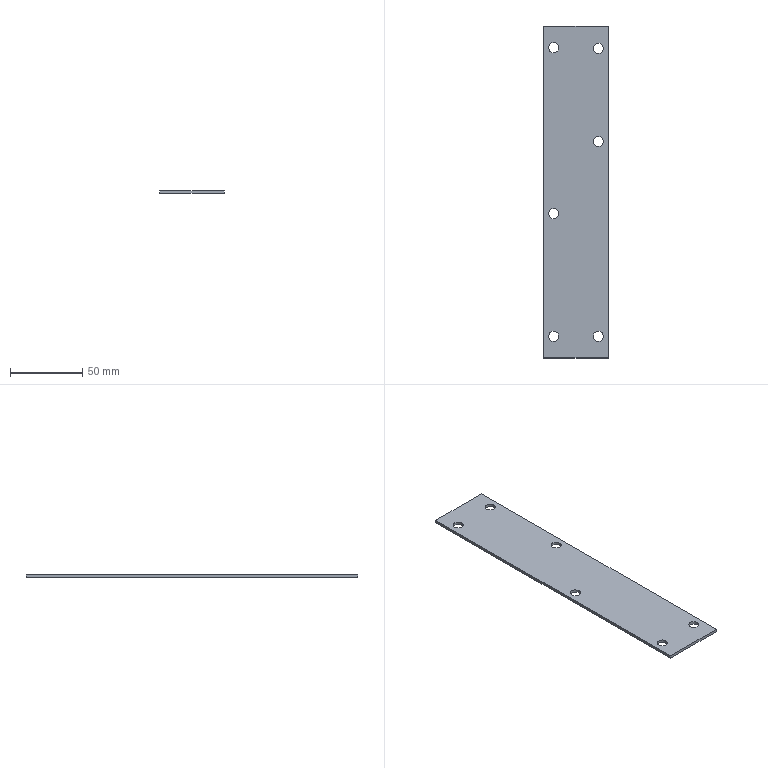Part | STEP file | 1_id1302_x_t | 1 solid | 18 faces | box 45 x 230 x 2 mm | volume 20238 mm3 | cylinder 12 | plane 6 | commonest cylinder face diameters 7 x12